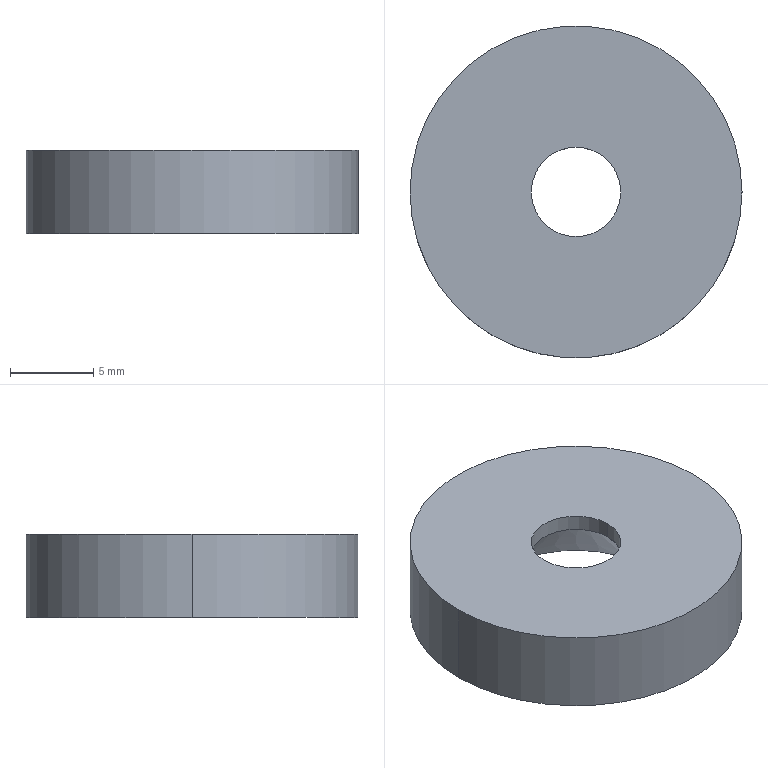Part | Creo | 1 solid | 8 faces | box 20 x 20 x 5 mm | volume 1284 mm3 | cylinder 4 | plane 2 | cone 2 | commonest cylinder face diameters 5.4 x2 20 x2
STEP:
#1=CARTESIAN_POINT('',(0.,0.,0.));
#2=DIRECTION('',(0.,0.,1.));
#3=DIRECTION('',(1.,0.,0.));
#4=AXIS2_PLACEMENT_3D('',#1,#2,#3);
#5=CARTESIAN_POINT('',(-243.201,282.071,-28.441));
#6=VERTEX_POINT('',#5);
#7=CARTESIAN_POINT('',(-263.201,282.071,-28.441));
#8=VERTEX_POINT('',#7);
#9=CARTESIAN_POINT('',(-253.201,282.071,-28.441));
#10=DIRECTION('',(0.,0.,-1.));
#11=DIRECTION('',(1.,0.,0.));
#12=AXIS2_PLACEMENT_3D('',#9,#10,#11);
#13=CIRCLE('',#12,10.);
#14=EDGE_CURVE('',#6,#8,#13,.T.);
#15=ORIENTED_EDGE('',*,*,#14,.F.);
#16=CARTESIAN_POINT('',(-253.201,282.071,-28.441));
#17=DIRECTION('',(0.,0.,-1.));
#18=DIRECTION('',(-1.,0.,0.));
#19=AXIS2_PLACEMENT_3D('',#16,#17,#18);
#20=CIRCLE('',#19,10.);
#21=EDGE_CURVE('',#8,#6,#20,.T.);
#22=ORIENTED_EDGE('',*,*,#21,.F.);
#23=EDGE_LOOP('',(#15,#22));
#24=FACE_OUTER_BOUND('',#23,.F.);
#25=CARTESIAN_POINT('',(-259.409,282.071,-28.441));
#26=VERTEX_POINT('',#25);
#27=CARTESIAN_POINT('',(-246.992,282.071,-28.441));
#28=VERTEX_POINT('',#27);
#29=CARTESIAN_POINT('',(-253.201,282.071,-28.441));
#30=DIRECTION('',(0.,0.,1.));
#31=DIRECTION('',(-1.,0.,0.));
#32=AXIS2_PLACEMENT_3D('',#29,#30,#31);
#33=CIRCLE('',#32,6.209);
#34=EDGE_CURVE('',#26,#28,#33,.T.);
#35=ORIENTED_EDGE('',*,*,#34,.F.);
#36=CARTESIAN_POINT('',(-253.201,282.071,-28.441));
#37=DIRECTION('',(0.,0.,1.));
#38=DIRECTION('',(1.,0.,0.));
#39=AXIS2_PLACEMENT_3D('',#36,#37,#38);
#40=CIRCLE('',#39,6.209);
#41=EDGE_CURVE('',#28,#26,#40,.T.);
#42=ORIENTED_EDGE('',*,*,#41,.F.);
#43=EDGE_LOOP('',(#35,#42));
#44=FACE_BOUND('',#43,.F.);
#45=CARTESIAN_POINT('',(-253.201,282.071,-28.441));
#46=DIRECTION('',(0.,0.,-1.));
#47=DIRECTION('',(-1.,0.,0.));
#48=AXIS2_PLACEMENT_3D('',#45,#46,#47);
#49=PLANE('',#48);
#50=ADVANCED_FACE('',(#24,#44),#49,.T.);
#51=CARTESIAN_POINT('',(-255.901,282.071,-24.405));
#52=VERTEX_POINT('',#51);
#53=CARTESIAN_POINT('',(-250.501,282.071,-24.405));
#54=VERTEX_POINT('',#53);
#55=CARTESIAN_POINT('',(-253.201,282.071,-24.405));
#56=DIRECTION('',(0.,0.,1.));
#57=DIRECTION('',(-1.,0.,0.));
#58=AXIS2_PLACEMENT_3D('',#55,#56,#57);
#59=CIRCLE('',#58,2.7);
#60=EDGE_CURVE('',#52,#54,#59,.T.);
#61=ORIENTED_EDGE('',*,*,#60,.F.);
#62=CARTESIAN_POINT('',(-255.901,282.071,-24.405));
#63=DIRECTION('',(-0.6561,0.,-0.7547));
#64=VECTOR('',#63,5.348);
#65=LINE('',#62,#64);
#66=EDGE_CURVE('',#52,#26,#65,.T.);
#67=ORIENTED_EDGE('',*,*,#66,.T.);
#68=ORIENTED_EDGE('',*,*,#34,.T.);
#69=CARTESIAN_POINT('',(-250.501,282.071,-24.405));
#70=DIRECTION('',(0.6561,0.,-0.7547));
#71=VECTOR('',#70,5.348);
#72=LINE('',#69,#71);
#73=EDGE_CURVE('',#54,#28,#72,.T.);
#74=ORIENTED_EDGE('',*,*,#73,.F.);
#75=EDGE_LOOP('',(#61,#67,#68,#74));
#76=FACE_OUTER_BOUND('',#75,.F.);
#77=CARTESIAN_POINT('',(-253.201,282.071,-26.423));
#78=DIRECTION('',(0.,0.,-1.));
#79=DIRECTION('',(-1.,0.,0.));
#80=AXIS2_PLACEMENT_3D('',#77,#78,#79);
#81=CONICAL_SURFACE('',#80,4.454,41.);
#82=ADVANCED_FACE('',(#76),#81,.F.);
#83=CARTESIAN_POINT('',(-250.501,282.071,-23.441));
#84=VERTEX_POINT('',#83);
#85=CARTESIAN_POINT('',(-255.901,282.071,-23.441));
#86=VERTEX_POINT('',#85);
#87=CARTESIAN_POINT('',(-253.201,282.071,-23.441));
#88=DIRECTION('',(0.,0.,-1.));
#89=DIRECTION('',(1.,0.,0.));
#90=AXIS2_PLACEMENT_3D('',#87,#88,#89);
#91=CIRCLE('',#90,2.7);
#92=EDGE_CURVE('',#84,#86,#91,.T.);
#93=ORIENTED_EDGE('',*,*,#92,.T.);
#94=CARTESIAN_POINT('',(-255.901,282.071,-23.441));
#95=DIRECTION('',(0.,0.,-1.));
#96=VECTOR('',#95,0.9639);
#97=LINE('',#94,#96);
#98=EDGE_CURVE('',#86,#52,#97,.T.);
#99=ORIENTED_EDGE('',*,*,#98,.T.);
#100=ORIENTED_EDGE('',*,*,#60,.T.);
#101=CARTESIAN_POINT('',(-250.501,282.071,-23.441));
#102=DIRECTION('',(0.,0.,-1.));
#103=VECTOR('',#102,0.9639);
#104=LINE('',#101,#103);
#105=EDGE_CURVE('',#84,#54,#104,.T.);
#106=ORIENTED_EDGE('',*,*,#105,.F.);
#107=EDGE_LOOP('',(#93,#99,#100,#106));
#108=FACE_OUTER_BOUND('',#107,.F.);
#109=CARTESIAN_POINT('',(-253.201,282.071,-23.441));
#110=DIRECTION('',(0.,0.,-1.));
#111=DIRECTION('',(-1.,0.,0.));
#112=AXIS2_PLACEMENT_3D('',#109,#110,#111);
#113=CYLINDRICAL_SURFACE('',#112,2.7);
#114=ADVANCED_FACE('',(#108),#113,.F.);
#115=CARTESIAN_POINT('',(-263.201,282.071,-23.441));
#116=VERTEX_POINT('',#115);
#117=CARTESIAN_POINT('',(-243.201,282.071,-23.441));
#118=VERTEX_POINT('',#117);
#119=CARTESIAN_POINT('',(-253.201,282.071,-23.441));
#120=DIRECTION('',(0.,0.,1.));
#121=DIRECTION('',(-1.,0.,0.));
#122=AXIS2_PLACEMENT_3D('',#119,#120,#121);
#123=CIRCLE('',#122,10.);
#124=EDGE_CURVE('',#116,#118,#123,.T.);
#125=ORIENTED_EDGE('',*,*,#124,.F.);
#126=CARTESIAN_POINT('',(-253.201,282.071,-23.441));
#127=DIRECTION('',(0.,0.,1.));
#128=DIRECTION('',(1.,0.,0.));
#129=AXIS2_PLACEMENT_3D('',#126,#127,#128);
#130=CIRCLE('',#129,10.);
#131=EDGE_CURVE('',#118,#116,#130,.T.);
#132=ORIENTED_EDGE('',*,*,#131,.F.);
#133=EDGE_LOOP('',(#125,#132));
#134=FACE_OUTER_BOUND('',#133,.F.);
#135=ORIENTED_EDGE('',*,*,#92,.F.);
#136=CARTESIAN_POINT('',(-253.201,282.071,-23.441));
#137=DIRECTION('',(0.,0.,-1.));
#138=DIRECTION('',(-1.,0.,0.));
#139=AXIS2_PLACEMENT_3D('',#136,#137,#138);
#140=CIRCLE('',#139,2.7);
#141=EDGE_CURVE('',#86,#84,#140,.T.);
#142=ORIENTED_EDGE('',*,*,#141,.F.);
#143=EDGE_LOOP('',(#135,#142));
#144=FACE_BOUND('',#143,.F.);
#145=CARTESIAN_POINT('',(-253.201,282.071,-23.441));
#146=DIRECTION('',(0.,0.,1.));
#147=DIRECTION('',(1.,0.,0.));
#148=AXIS2_PLACEMENT_3D('',#145,#146,#147);
#149=PLANE('',#148);
#150=ADVANCED_FACE('',(#134,#144),#149,.T.);
#151=ORIENTED_EDGE('',*,*,#141,.T.);
#152=ORIENTED_EDGE('',*,*,#105,.T.);
#153=CARTESIAN_POINT('',(-253.201,282.071,-24.405));
#154=DIRECTION('',(0.,0.,1.));
#155=DIRECTION('',(1.,0.,0.));
#156=AXIS2_PLACEMENT_3D('',#153,#154,#155);
#157=CIRCLE('',#156,2.7);
#158=EDGE_CURVE('',#54,#52,#157,.T.);
#159=ORIENTED_EDGE('',*,*,#158,.T.);
#160=ORIENTED_EDGE('',*,*,#98,.F.);
#161=EDGE_LOOP('',(#151,#152,#159,#160));
#162=FACE_OUTER_BOUND('',#161,.F.);
#163=CARTESIAN_POINT('',(-253.201,282.071,-23.441));
#164=DIRECTION('',(0.,0.,-1.));
#165=DIRECTION('',(-1.,0.,0.));
#166=AXIS2_PLACEMENT_3D('',#163,#164,#165);
#167=CYLINDRICAL_SURFACE('',#166,2.7);
#168=ADVANCED_FACE('',(#162),#167,.F.);
#169=ORIENTED_EDGE('',*,*,#158,.F.);
#170=ORIENTED_EDGE('',*,*,#73,.T.);
#171=ORIENTED_EDGE('',*,*,#41,.T.);
#172=ORIENTED_EDGE('',*,*,#66,.F.);
#173=EDGE_LOOP('',(#169,#170,#171,#172));
#174=FACE_OUTER_BOUND('',#173,.F.);
#175=CARTESIAN_POINT('',(-253.201,282.071,-26.423));
#176=DIRECTION('',(0.,0.,-1.));
#177=DIRECTION('',(-1.,0.,0.));
#178=AXIS2_PLACEMENT_3D('',#175,#176,#177);
#179=CONICAL_SURFACE('',#178,4.454,41.);
#180=ADVANCED_FACE('',(#174),#179,.F.);
#181=ORIENTED_EDGE('',*,*,#14,.T.);
#182=CARTESIAN_POINT('',(-263.201,282.071,-23.441));
#183=DIRECTION('',(0.,0.,-1.));
#184=VECTOR('',#183,5.);
#185=LINE('',#182,#184);
#186=EDGE_CURVE('',#116,#8,#185,.T.);
#187=ORIENTED_EDGE('',*,*,#186,.F.);
#188=ORIENTED_EDGE('',*,*,#124,.T.);
#189=CARTESIAN_POINT('',(-243.201,282.071,-23.441));
#190=DIRECTION('',(0.,0.,-1.));
#191=VECTOR('',#190,5.);
#192=LINE('',#189,#191);
#193=EDGE_CURVE('',#118,#6,#192,.T.);
#194=ORIENTED_EDGE('',*,*,#193,.T.);
#195=EDGE_LOOP('',(#181,#187,#188,#194));
#196=FACE_OUTER_BOUND('',#195,.F.);
#197=CARTESIAN_POINT('',(-253.201,282.071,-23.441));
#198=DIRECTION('',(0.,0.,-1.));
#199=DIRECTION('',(-1.,0.,0.));
#200=AXIS2_PLACEMENT_3D('',#197,#198,#199);
#201=CYLINDRICAL_SURFACE('',#200,10.);
#202=ADVANCED_FACE('',(#196),#201,.T.);
#203=ORIENTED_EDGE('',*,*,#21,.T.);
#204=ORIENTED_EDGE('',*,*,#193,.F.);
#205=ORIENTED_EDGE('',*,*,#131,.T.);
#206=ORIENTED_EDGE('',*,*,#186,.T.);
#207=EDGE_LOOP('',(#203,#204,#205,#206));
#208=FACE_OUTER_BOUND('',#207,.F.);
#209=CARTESIAN_POINT('',(-253.201,282.071,-23.441));
#210=DIRECTION('',(0.,0.,-1.));
#211=DIRECTION('',(-1.,0.,0.));
#212=AXIS2_PLACEMENT_3D('',#209,#210,#211);
#213=CYLINDRICAL_SURFACE('',#212,10.);
#214=ADVANCED_FACE('',(#208),#213,.T.);
#215=CLOSED_SHELL('',(#50,#82,#114,#150,#168,#180,#202,#214));
#216=MANIFOLD_SOLID_BREP('',#215);
#217=(LENGTH_UNIT()NAMED_UNIT(*)SI_UNIT(.MILLI.,.METRE.));
#218=UNCERTAINTY_MEASURE_WITH_UNIT(LENGTH_MEASURE(0.002873),#217,'','');
#219=(NAMED_UNIT(*)PLANE_ANGLE_UNIT()SI_UNIT($,.RADIAN.));
#220=PLANE_ANGLE_MEASURE_WITH_UNIT(PLANE_ANGLE_MEASURE(0.01745),#219);
#221=(CONVERSION_BASED_UNIT('DEGREE',#220)NAMED_UNIT(*)PLANE_ANGLE_UNIT());
#222=(NAMED_UNIT(*)SI_UNIT($,.STERADIAN.)SOLID_ANGLE_UNIT());
#223=(GEOMETRIC_REPRESENTATION_CONTEXT(3)GLOBAL_UNCERTAINTY_ASSIGNED_CONTEXT((#218))GLOBAL_UNIT_ASSIGNED_CONTEXT((#217,#221,#222))REPRESENTATION_CONTEXT('',''));
#224=ADVANCED_BREP_SHAPE_REPRESENTATION('',(#4,#216),#223);